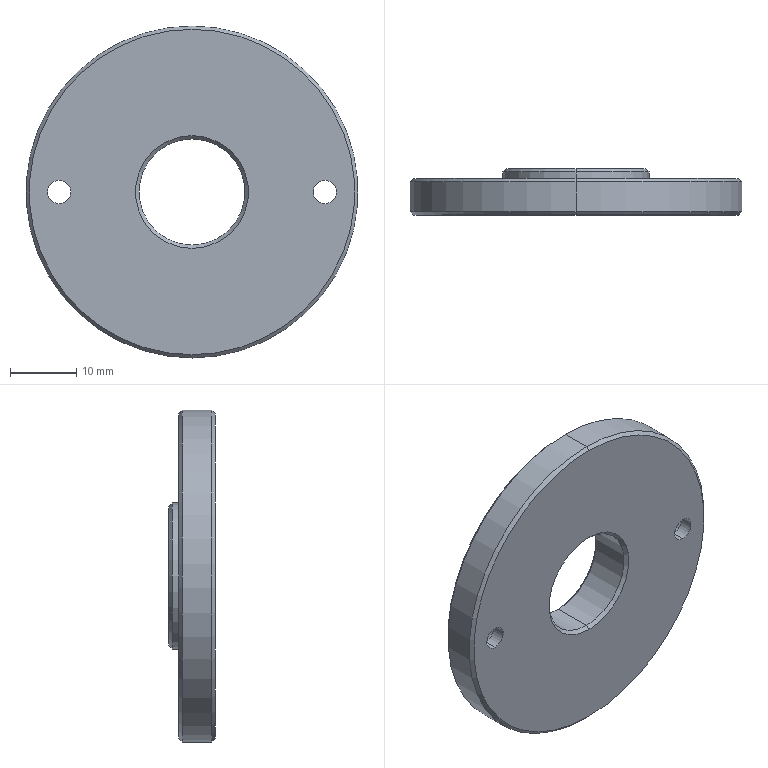Part | SolidWorks | features 3DProfileFeature 1, Chamfer 1, HoleWzd 1, Revolution 1 | 1 solid | 29 faces | box 50 x 7 x 50 mm | volume 9665 mm3 | cylinder 14 | cone 10 | plane 5 | commonest cylinder face diameters 3.5 x4 6 x4 16 x2 22 x2 50 x2
STEP:
#1=CARTESIAN_POINT('',(0.,0.5,8.));
#2=VERTEX_POINT('',#1);
#3=CARTESIAN_POINT('',(0.,0.5,-8.));
#4=VERTEX_POINT('',#3);
#5=CARTESIAN_POINT('',(0.,0.5,0.));
#6=DIRECTION('',(0.,-1.,0.));
#7=DIRECTION('',(0.,0.,1.));
#8=AXIS2_PLACEMENT_3D('',#5,#6,#7);
#9=CIRCLE('',#8,8.);
#10=EDGE_CURVE('',#2,#4,#9,.T.);
#11=ORIENTED_EDGE('',*,*,#10,.F.);
#12=CARTESIAN_POINT('',(0.,0.,8.5));
#13=VERTEX_POINT('',#12);
#14=CARTESIAN_POINT('',(0.,0.,8.5));
#15=DIRECTION('',(0.,-0.7071,0.7071));
#16=VECTOR('',#15,1000.);
#17=LINE('',#14,#16);
#18=EDGE_CURVE('',#2,#13,#17,.T.);
#19=ORIENTED_EDGE('',*,*,#18,.T.);
#20=CARTESIAN_POINT('',(0.,0.,-8.5));
#21=VERTEX_POINT('',#20);
#22=CARTESIAN_POINT('',(0.,0.,0.));
#23=DIRECTION('',(0.,1.,0.));
#24=DIRECTION('',(0.,0.,1.));
#25=AXIS2_PLACEMENT_3D('',#22,#23,#24);
#26=CIRCLE('',#25,8.5);
#27=EDGE_CURVE('',#21,#13,#26,.T.);
#28=ORIENTED_EDGE('',*,*,#27,.F.);
#29=CARTESIAN_POINT('',(0.,0.,-8.5));
#30=DIRECTION('',(0.,-0.7071,-0.7071));
#31=VECTOR('',#30,1000.);
#32=LINE('',#29,#31);
#33=EDGE_CURVE('',#4,#21,#32,.T.);
#34=ORIENTED_EDGE('',*,*,#33,.F.);
#35=EDGE_LOOP('',(#11,#19,#28,#34));
#36=FACE_OUTER_BOUND('',#35,.T.);
#37=CARTESIAN_POINT('',(0.,0.,0.));
#38=DIRECTION('',(0.,-1.,0.));
#39=DIRECTION('',(0.,0.,-1.));
#40=AXIS2_PLACEMENT_3D('',#37,#38,#39);
#41=CONICAL_SURFACE('',#40,8.5,0.7854);
#42=ADVANCED_FACE('',(#36),#41,.F.);
#43=CARTESIAN_POINT('',(0.,6.5,-8.));
#44=VERTEX_POINT('',#43);
#45=CARTESIAN_POINT('',(0.,6.5,8.));
#46=VERTEX_POINT('',#45);
#47=CARTESIAN_POINT('',(0.,6.5,0.));
#48=DIRECTION('',(0.,1.,0.));
#49=DIRECTION('',(0.,0.,-1.));
#50=AXIS2_PLACEMENT_3D('',#47,#48,#49);
#51=CIRCLE('',#50,8.);
#52=EDGE_CURVE('',#44,#46,#51,.T.);
#53=ORIENTED_EDGE('',*,*,#52,.F.);
#54=CARTESIAN_POINT('',(0.,7.,-8.5));
#55=VERTEX_POINT('',#54);
#56=CARTESIAN_POINT('',(0.,6.5,-8.));
#57=DIRECTION('',(0.,0.7071,-0.7071));
#58=VECTOR('',#57,1000.);
#59=LINE('',#56,#58);
#60=EDGE_CURVE('',#44,#55,#59,.T.);
#61=ORIENTED_EDGE('',*,*,#60,.T.);
#62=CARTESIAN_POINT('',(0.,7.,8.5));
#63=VERTEX_POINT('',#62);
#64=CARTESIAN_POINT('',(0.,7.,0.));
#65=DIRECTION('',(0.,-1.,0.));
#66=DIRECTION('',(0.,0.,-1.));
#67=AXIS2_PLACEMENT_3D('',#64,#65,#66);
#68=CIRCLE('',#67,8.5);
#69=EDGE_CURVE('',#63,#55,#68,.T.);
#70=ORIENTED_EDGE('',*,*,#69,.F.);
#71=CARTESIAN_POINT('',(0.,6.5,8.));
#72=DIRECTION('',(0.,0.7071,0.7071));
#73=VECTOR('',#72,1000.);
#74=LINE('',#71,#73);
#75=EDGE_CURVE('',#46,#63,#74,.T.);
#76=ORIENTED_EDGE('',*,*,#75,.F.);
#77=EDGE_LOOP('',(#53,#61,#70,#76));
#78=FACE_OUTER_BOUND('',#77,.T.);
#79=CARTESIAN_POINT('',(0.,6.5,0.));
#80=DIRECTION('',(0.,1.,0.));
#81=DIRECTION('',(0.,0.,1.));
#82=AXIS2_PLACEMENT_3D('',#79,#80,#81);
#83=CONICAL_SURFACE('',#82,8.,0.7854);
#84=ADVANCED_FACE('',(#78),#83,.F.);
#85=CARTESIAN_POINT('',(0.,7.,10.5));
#86=VERTEX_POINT('',#85);
#87=CARTESIAN_POINT('',(0.,7.,-10.5));
#88=VERTEX_POINT('',#87);
#89=CARTESIAN_POINT('',(0.,7.,0.));
#90=DIRECTION('',(0.,1.,0.));
#91=DIRECTION('',(0.,0.,-1.));
#92=AXIS2_PLACEMENT_3D('',#89,#90,#91);
#93=CIRCLE('',#92,10.5);
#94=EDGE_CURVE('',#86,#88,#93,.T.);
#95=ORIENTED_EDGE('',*,*,#94,.F.);
#96=CARTESIAN_POINT('',(0.,6.5,11.));
#97=VERTEX_POINT('',#96);
#98=CARTESIAN_POINT('',(0.,7.,10.5));
#99=DIRECTION('',(0.,-0.7071,0.7071));
#100=VECTOR('',#99,1000.);
#101=LINE('',#98,#100);
#102=EDGE_CURVE('',#86,#97,#101,.T.);
#103=ORIENTED_EDGE('',*,*,#102,.T.);
#104=CARTESIAN_POINT('',(0.,6.5,-11.));
#105=VERTEX_POINT('',#104);
#106=CARTESIAN_POINT('',(0.,6.5,0.));
#107=DIRECTION('',(0.,-1.,0.));
#108=DIRECTION('',(0.,0.,-1.));
#109=AXIS2_PLACEMENT_3D('',#106,#107,#108);
#110=CIRCLE('',#109,11.);
#111=EDGE_CURVE('',#105,#97,#110,.T.);
#112=ORIENTED_EDGE('',*,*,#111,.F.);
#113=CARTESIAN_POINT('',(0.,7.,-10.5));
#114=DIRECTION('',(0.,-0.7071,-0.7071));
#115=VECTOR('',#114,1000.);
#116=LINE('',#113,#115);
#117=EDGE_CURVE('',#88,#105,#116,.T.);
#118=ORIENTED_EDGE('',*,*,#117,.F.);
#119=EDGE_LOOP('',(#95,#103,#112,#118));
#120=FACE_OUTER_BOUND('',#119,.T.);
#121=CARTESIAN_POINT('',(0.,7.,0.));
#122=DIRECTION('',(0.,-1.,0.));
#123=DIRECTION('',(0.,0.,-1.));
#124=AXIS2_PLACEMENT_3D('',#121,#122,#123);
#125=CONICAL_SURFACE('',#124,10.5,0.7854);
#126=ADVANCED_FACE('',(#120),#125,.T.);
#127=CARTESIAN_POINT('',(0.,5.5,24.5));
#128=VERTEX_POINT('',#127);
#129=CARTESIAN_POINT('',(0.,5.5,-24.5));
#130=VERTEX_POINT('',#129);
#131=CARTESIAN_POINT('',(0.,5.5,0.));
#132=DIRECTION('',(0.,1.,0.));
#133=DIRECTION('',(0.,0.,-1.));
#134=AXIS2_PLACEMENT_3D('',#131,#132,#133);
#135=CIRCLE('',#134,24.5);
#136=EDGE_CURVE('',#128,#130,#135,.T.);
#137=ORIENTED_EDGE('',*,*,#136,.F.);
#138=CARTESIAN_POINT('',(0.,5.,25.));
#139=VERTEX_POINT('',#138);
#140=CARTESIAN_POINT('',(0.,5.5,24.5));
#141=DIRECTION('',(0.,-0.7071,0.7071));
#142=VECTOR('',#141,1000.);
#143=LINE('',#140,#142);
#144=EDGE_CURVE('',#128,#139,#143,.T.);
#145=ORIENTED_EDGE('',*,*,#144,.T.);
#146=CARTESIAN_POINT('',(0.,5.,-25.));
#147=VERTEX_POINT('',#146);
#148=CARTESIAN_POINT('',(0.,5.,0.));
#149=DIRECTION('',(0.,-1.,0.));
#150=DIRECTION('',(0.,0.,-1.));
#151=AXIS2_PLACEMENT_3D('',#148,#149,#150);
#152=CIRCLE('',#151,25.);
#153=EDGE_CURVE('',#147,#139,#152,.T.);
#154=ORIENTED_EDGE('',*,*,#153,.F.);
#155=CARTESIAN_POINT('',(0.,5.5,-24.5));
#156=DIRECTION('',(0.,-0.7071,-0.7071));
#157=VECTOR('',#156,1000.);
#158=LINE('',#155,#157);
#159=EDGE_CURVE('',#130,#147,#158,.T.);
#160=ORIENTED_EDGE('',*,*,#159,.F.);
#161=EDGE_LOOP('',(#137,#145,#154,#160));
#162=FACE_OUTER_BOUND('',#161,.T.);
#163=CARTESIAN_POINT('',(0.,5.5,0.));
#164=DIRECTION('',(0.,-1.,0.));
#165=DIRECTION('',(0.,0.,-1.));
#166=AXIS2_PLACEMENT_3D('',#163,#164,#165);
#167=CONICAL_SURFACE('',#166,24.5,0.7854);
#168=ADVANCED_FACE('',(#162),#167,.T.);
#169=CARTESIAN_POINT('',(0.,0.,-24.5));
#170=VERTEX_POINT('',#169);
#171=CARTESIAN_POINT('',(0.,0.,24.5));
#172=VERTEX_POINT('',#171);
#173=CARTESIAN_POINT('',(0.,0.,0.));
#174=DIRECTION('',(0.,-1.,0.));
#175=DIRECTION('',(0.,0.,1.));
#176=AXIS2_PLACEMENT_3D('',#173,#174,#175);
#177=CIRCLE('',#176,24.5);
#178=EDGE_CURVE('',#170,#172,#177,.T.);
#179=ORIENTED_EDGE('',*,*,#178,.F.);
#180=CARTESIAN_POINT('',(0.,0.5,-25.));
#181=VERTEX_POINT('',#180);
#182=CARTESIAN_POINT('',(0.,0.5,-25.));
#183=DIRECTION('',(0.,0.7071,-0.7071));
#184=VECTOR('',#183,1000.);
#185=LINE('',#182,#184);
#186=EDGE_CURVE('',#170,#181,#185,.T.);
#187=ORIENTED_EDGE('',*,*,#186,.T.);
#188=CARTESIAN_POINT('',(0.,0.5,25.));
#189=VERTEX_POINT('',#188);
#190=CARTESIAN_POINT('',(0.,0.5,0.));
#191=DIRECTION('',(0.,1.,0.));
#192=DIRECTION('',(0.,0.,1.));
#193=AXIS2_PLACEMENT_3D('',#190,#191,#192);
#194=CIRCLE('',#193,25.);
#195=EDGE_CURVE('',#189,#181,#194,.T.);
#196=ORIENTED_EDGE('',*,*,#195,.F.);
#197=CARTESIAN_POINT('',(0.,0.5,25.));
#198=DIRECTION('',(0.,0.7071,0.7071));
#199=VECTOR('',#198,1000.);
#200=LINE('',#197,#199);
#201=EDGE_CURVE('',#172,#189,#200,.T.);
#202=ORIENTED_EDGE('',*,*,#201,.F.);
#203=EDGE_LOOP('',(#179,#187,#196,#202));
#204=FACE_OUTER_BOUND('',#203,.T.);
#205=CARTESIAN_POINT('',(0.,0.5,0.));
#206=DIRECTION('',(0.,1.,0.));
#207=DIRECTION('',(0.,0.,1.));
#208=AXIS2_PLACEMENT_3D('',#205,#206,#207);
#209=CONICAL_SURFACE('',#208,25.,0.7854);
#210=ADVANCED_FACE('',(#204),#209,.T.);
#211=CARTESIAN_POINT('',(-20.,2.,-3.));
#212=VERTEX_POINT('',#211);
#213=CARTESIAN_POINT('',(-20.,2.,3.));
#214=VERTEX_POINT('',#213);
#215=CARTESIAN_POINT('',(-20.,2.,0.));
#216=DIRECTION('',(0.,1.,0.));
#217=DIRECTION('',(0.,0.,1.));
#218=AXIS2_PLACEMENT_3D('',#215,#216,#217);
#219=CIRCLE('',#218,3.);
#220=EDGE_CURVE('',#212,#214,#219,.T.);
#221=ORIENTED_EDGE('',*,*,#220,.F.);
#222=CARTESIAN_POINT('',(-20.,5.5,-3.));
#223=VERTEX_POINT('',#222);
#224=CARTESIAN_POINT('',(-20.,5.5,-3.));
#225=DIRECTION('',(0.,1.,0.));
#226=VECTOR('',#225,1000.);
#227=LINE('',#224,#226);
#228=EDGE_CURVE('',#212,#223,#227,.T.);
#229=ORIENTED_EDGE('',*,*,#228,.T.);
#230=CARTESIAN_POINT('',(-20.,5.5,3.));
#231=VERTEX_POINT('',#230);
#232=CARTESIAN_POINT('',(-20.,5.5,0.));
#233=DIRECTION('',(0.,1.,0.));
#234=DIRECTION('',(0.,0.,1.));
#235=AXIS2_PLACEMENT_3D('',#232,#233,#234);
#236=CIRCLE('',#235,3.);
#237=EDGE_CURVE('',#223,#231,#236,.T.);
#238=ORIENTED_EDGE('',*,*,#237,.T.);
#239=CARTESIAN_POINT('',(-20.,5.5,3.));
#240=DIRECTION('',(0.,1.,0.));
#241=VECTOR('',#240,1000.);
#242=LINE('',#239,#241);
#243=EDGE_CURVE('',#214,#231,#242,.T.);
#244=ORIENTED_EDGE('',*,*,#243,.F.);
#245=EDGE_LOOP('',(#221,#229,#238,#244));
#246=FACE_OUTER_BOUND('',#245,.T.);
#247=CARTESIAN_POINT('',(-20.,5.5,0.));
#248=DIRECTION('',(0.,1.,0.));
#249=DIRECTION('',(0.,0.,1.));
#250=AXIS2_PLACEMENT_3D('',#247,#248,#249);
#251=CYLINDRICAL_SURFACE('',#250,3.);
#252=ADVANCED_FACE('',(#246),#251,.F.);
#253=CARTESIAN_POINT('',(-20.,0.,-1.75));
#254=VERTEX_POINT('',#253);
#255=CARTESIAN_POINT('',(-20.,0.,1.75));
#256=VERTEX_POINT('',#255);
#257=CARTESIAN_POINT('',(-20.,0.,0.));
#258=DIRECTION('',(0.,1.,0.));
#259=DIRECTION('',(0.,0.,1.));
#260=AXIS2_PLACEMENT_3D('',#257,#258,#259);
#261=CIRCLE('',#260,1.75);
#262=EDGE_CURVE('',#254,#256,#261,.T.);
#263=ORIENTED_EDGE('',*,*,#262,.F.);
#264=CARTESIAN_POINT('',(-20.,2.,-1.75));
#265=VERTEX_POINT('',#264);
#266=CARTESIAN_POINT('',(-20.,5.5,-1.75));
#267=DIRECTION('',(0.,1.,0.));
#268=VECTOR('',#267,1000.);
#269=LINE('',#266,#268);
#270=EDGE_CURVE('',#254,#265,#269,.T.);
#271=ORIENTED_EDGE('',*,*,#270,.T.);
#272=CARTESIAN_POINT('',(-20.,2.,1.75));
#273=VERTEX_POINT('',#272);
#274=CARTESIAN_POINT('',(-20.,2.,0.));
#275=DIRECTION('',(0.,1.,0.));
#276=DIRECTION('',(0.,0.,1.));
#277=AXIS2_PLACEMENT_3D('',#274,#275,#276);
#278=CIRCLE('',#277,1.75);
#279=EDGE_CURVE('',#265,#273,#278,.T.);
#280=ORIENTED_EDGE('',*,*,#279,.T.);
#281=CARTESIAN_POINT('',(-20.,5.5,1.75));
#282=DIRECTION('',(0.,1.,0.));
#283=VECTOR('',#282,1000.);
#284=LINE('',#281,#283);
#285=EDGE_CURVE('',#256,#273,#284,.T.);
#286=ORIENTED_EDGE('',*,*,#285,.F.);
#287=EDGE_LOOP('',(#263,#271,#280,#286));
#288=FACE_OUTER_BOUND('',#287,.T.);
#289=CARTESIAN_POINT('',(-20.,5.5,0.));
#290=DIRECTION('',(0.,1.,0.));
#291=DIRECTION('',(0.,0.,1.));
#292=AXIS2_PLACEMENT_3D('',#289,#290,#291);
#293=CYLINDRICAL_SURFACE('',#292,1.75);
#294=ADVANCED_FACE('',(#288),#293,.F.);
#295=CARTESIAN_POINT('',(20.,2.,-3.));
#296=VERTEX_POINT('',#295);
#297=CARTESIAN_POINT('',(20.,2.,3.));
#298=VERTEX_POINT('',#297);
#299=CARTESIAN_POINT('',(20.,2.,0.));
#300=DIRECTION('',(0.,1.,0.));
#301=DIRECTION('',(0.,0.,1.));
#302=AXIS2_PLACEMENT_3D('',#299,#300,#301);
#303=CIRCLE('',#302,3.);
#304=EDGE_CURVE('',#296,#298,#303,.T.);
#305=ORIENTED_EDGE('',*,*,#304,.F.);
#306=CARTESIAN_POINT('',(20.,5.5,-3.));
#307=VERTEX_POINT('',#306);
#308=CARTESIAN_POINT('',(20.,5.5,-3.));
#309=DIRECTION('',(0.,1.,0.));
#310=VECTOR('',#309,1000.);
#311=LINE('',#308,#310);
#312=EDGE_CURVE('',#296,#307,#311,.T.);
#313=ORIENTED_EDGE('',*,*,#312,.T.);
#314=CARTESIAN_POINT('',(20.,5.5,3.));
#315=VERTEX_POINT('',#314);
#316=CARTESIAN_POINT('',(20.,5.5,0.));
#317=DIRECTION('',(0.,1.,0.));
#318=DIRECTION('',(0.,0.,1.));
#319=AXIS2_PLACEMENT_3D('',#316,#317,#318);
#320=CIRCLE('',#319,3.);
#321=EDGE_CURVE('',#307,#315,#320,.T.);
#322=ORIENTED_EDGE('',*,*,#321,.T.);
#323=CARTESIAN_POINT('',(20.,5.5,3.));
#324=DIRECTION('',(0.,1.,0.));
#325=VECTOR('',#324,1000.);
#326=LINE('',#323,#325);
#327=EDGE_CURVE('',#298,#315,#326,.T.);
#328=ORIENTED_EDGE('',*,*,#327,.F.);
#329=EDGE_LOOP('',(#305,#313,#322,#328));
#330=FACE_OUTER_BOUND('',#329,.T.);
#331=CARTESIAN_POINT('',(20.,5.5,0.));
#332=DIRECTION('',(0.,1.,0.));
#333=DIRECTION('',(0.,0.,1.));
#334=AXIS2_PLACEMENT_3D('',#331,#332,#333);
#335=CYLINDRICAL_SURFACE('',#334,3.);
#336=ADVANCED_FACE('',(#330),#335,.F.);
#337=CARTESIAN_POINT('',(20.,0.,-1.75));
#338=VERTEX_POINT('',#337);
#339=CARTESIAN_POINT('',(20.,0.,1.75));
#340=VERTEX_POINT('',#339);
#341=CARTESIAN_POINT('',(20.,0.,0.));
#342=DIRECTION('',(0.,1.,0.));
#343=DIRECTION('',(0.,0.,1.));
#344=AXIS2_PLACEMENT_3D('',#341,#342,#343);
#345=CIRCLE('',#344,1.75);
#346=EDGE_CURVE('',#338,#340,#345,.T.);
#347=ORIENTED_EDGE('',*,*,#346,.F.);
#348=CARTESIAN_POINT('',(20.,2.,-1.75));
#349=VERTEX_POINT('',#348);
#350=CARTESIAN_POINT('',(20.,5.5,-1.75));
#351=DIRECTION('',(0.,1.,0.));
#352=VECTOR('',#351,1000.);
#353=LINE('',#350,#352);
#354=EDGE_CURVE('',#338,#349,#353,.T.);
#355=ORIENTED_EDGE('',*,*,#354,.T.);
#356=CARTESIAN_POINT('',(20.,2.,1.75));
#357=VERTEX_POINT('',#356);
#358=CARTESIAN_POINT('',(20.,2.,0.));
#359=DIRECTION('',(0.,1.,0.));
#360=DIRECTION('',(0.,0.,1.));
#361=AXIS2_PLACEMENT_3D('',#358,#359,#360);
#362=CIRCLE('',#361,1.75);
#363=EDGE_CURVE('',#349,#357,#362,.T.);
#364=ORIENTED_EDGE('',*,*,#363,.T.);
#365=CARTESIAN_POINT('',(20.,5.5,1.75));
#366=DIRECTION('',(0.,1.,0.));
#367=VECTOR('',#366,1000.);
#368=LINE('',#365,#367);
#369=EDGE_CURVE('',#340,#357,#368,.T.);
#370=ORIENTED_EDGE('',*,*,#369,.F.);
#371=EDGE_LOOP('',(#347,#355,#364,#370));
#372=FACE_OUTER_BOUND('',#371,.T.);
#373=CARTESIAN_POINT('',(20.,5.5,0.));
#374=DIRECTION('',(0.,1.,0.));
#375=DIRECTION('',(0.,0.,1.));
#376=AXIS2_PLACEMENT_3D('',#373,#374,#375);
#377=CYLINDRICAL_SURFACE('',#376,1.75);
#378=ADVANCED_FACE('',(#372),#377,.F.);
#379=ORIENTED_EDGE('',*,*,#10,.T.);
#380=CARTESIAN_POINT('',(0.,21.458,-8.));
#381=DIRECTION('',(0.,1.,0.));
#382=VECTOR('',#381,1000.);
#383=LINE('',#380,#382);
#384=EDGE_CURVE('',#4,#44,#383,.T.);
#385=ORIENTED_EDGE('',*,*,#384,.T.);
#386=ORIENTED_EDGE('',*,*,#52,.T.);
#387=CARTESIAN_POINT('',(0.,21.458,8.));
#388=DIRECTION('',(0.,1.,0.));
#389=VECTOR('',#388,1000.);
#390=LINE('',#387,#389);
#391=EDGE_CURVE('',#2,#46,#390,.T.);
#392=ORIENTED_EDGE('',*,*,#391,.F.);
#393=EDGE_LOOP('',(#379,#385,#386,#392));
#394=FACE_OUTER_BOUND('',#393,.T.);
#395=CARTESIAN_POINT('',(0.,21.458,0.));
#396=DIRECTION('',(0.,1.,0.));
#397=DIRECTION('',(0.,0.,1.));
#398=AXIS2_PLACEMENT_3D('',#395,#396,#397);
#399=CYLINDRICAL_SURFACE('',#398,8.);
#400=ADVANCED_FACE('',(#394),#399,.F.);
#401=CARTESIAN_POINT('',(0.,5.5,11.));
#402=VERTEX_POINT('',#401);
#403=CARTESIAN_POINT('',(0.,5.5,-11.));
#404=VERTEX_POINT('',#403);
#405=CARTESIAN_POINT('',(0.,5.5,0.));
#406=DIRECTION('',(0.,1.,0.));
#407=DIRECTION('',(0.,0.,1.));
#408=AXIS2_PLACEMENT_3D('',#405,#406,#407);
#409=CIRCLE('',#408,11.);
#410=EDGE_CURVE('',#402,#404,#409,.T.);
#411=ORIENTED_EDGE('',*,*,#410,.T.);
#412=CARTESIAN_POINT('',(0.,21.458,-11.));
#413=DIRECTION('',(0.,1.,0.));
#414=VECTOR('',#413,1000.);
#415=LINE('',#412,#414);
#416=EDGE_CURVE('',#404,#105,#415,.T.);
#417=ORIENTED_EDGE('',*,*,#416,.T.);
#418=ORIENTED_EDGE('',*,*,#111,.T.);
#419=CARTESIAN_POINT('',(0.,21.458,11.));
#420=DIRECTION('',(0.,1.,0.));
#421=VECTOR('',#420,1000.);
#422=LINE('',#419,#421);
#423=EDGE_CURVE('',#402,#97,#422,.T.);
#424=ORIENTED_EDGE('',*,*,#423,.F.);
#425=EDGE_LOOP('',(#411,#417,#418,#424));
#426=FACE_OUTER_BOUND('',#425,.T.);
#427=CARTESIAN_POINT('',(0.,21.458,0.));
#428=DIRECTION('',(0.,1.,0.));
#429=DIRECTION('',(0.,0.,1.));
#430=AXIS2_PLACEMENT_3D('',#427,#428,#429);
#431=CYLINDRICAL_SURFACE('',#430,11.);
#432=ADVANCED_FACE('',(#426),#431,.T.);
#433=ORIENTED_EDGE('',*,*,#195,.T.);
#434=CARTESIAN_POINT('',(0.,21.458,-25.));
#435=DIRECTION('',(0.,1.,0.));
#436=VECTOR('',#435,1000.);
#437=LINE('',#434,#436);
#438=EDGE_CURVE('',#181,#147,#437,.T.);
#439=ORIENTED_EDGE('',*,*,#438,.T.);
#440=ORIENTED_EDGE('',*,*,#153,.T.);
#441=CARTESIAN_POINT('',(0.,21.458,25.));
#442=DIRECTION('',(0.,1.,0.));
#443=VECTOR('',#442,1000.);
#444=LINE('',#441,#443);
#445=EDGE_CURVE('',#189,#139,#444,.T.);
#446=ORIENTED_EDGE('',*,*,#445,.F.);
#447=EDGE_LOOP('',(#433,#439,#440,#446));
#448=FACE_OUTER_BOUND('',#447,.T.);
#449=CARTESIAN_POINT('',(0.,21.458,0.));
#450=DIRECTION('',(0.,1.,0.));
#451=DIRECTION('',(0.,0.,1.));
#452=AXIS2_PLACEMENT_3D('',#449,#450,#451);
#453=CYLINDRICAL_SURFACE('',#452,25.);
#454=ADVANCED_FACE('',(#448),#453,.T.);
#455=CARTESIAN_POINT('',(0.,5.5,0.));
#456=DIRECTION('',(0.,1.,0.));
#457=DIRECTION('',(0.,0.,-1.));
#458=AXIS2_PLACEMENT_3D('',#455,#456,#457);
#459=CIRCLE('',#458,24.5);
#460=EDGE_CURVE('',#130,#128,#459,.T.);
#461=ORIENTED_EDGE('',*,*,#460,.T.);
#462=ORIENTED_EDGE('',*,*,#136,.T.);
#463=EDGE_LOOP('',(#461,#462));
#464=FACE_OUTER_BOUND('',#463,.T.);
#465=ORIENTED_EDGE('',*,*,#410,.F.);
#466=CARTESIAN_POINT('',(0.,5.5,0.));
#467=DIRECTION('',(0.,1.,0.));
#468=DIRECTION('',(0.,0.,1.));
#469=AXIS2_PLACEMENT_3D('',#466,#467,#468);
#470=CIRCLE('',#469,11.);
#471=EDGE_CURVE('',#404,#402,#470,.T.);
#472=ORIENTED_EDGE('',*,*,#471,.F.);
#473=EDGE_LOOP('',(#465,#472));
#474=FACE_BOUND('',#473,.T.);
#475=CARTESIAN_POINT('',(20.,5.5,0.));
#476=DIRECTION('',(0.,1.,0.));
#477=DIRECTION('',(0.,0.,1.));
#478=AXIS2_PLACEMENT_3D('',#475,#476,#477);
#479=CIRCLE('',#478,3.);
#480=EDGE_CURVE('',#315,#307,#479,.T.);
#481=ORIENTED_EDGE('',*,*,#480,.F.);
#482=ORIENTED_EDGE('',*,*,#321,.F.);
#483=EDGE_LOOP('',(#481,#482));
#484=FACE_BOUND('',#483,.T.);
#485=CARTESIAN_POINT('',(-20.,5.5,0.));
#486=DIRECTION('',(0.,1.,0.));
#487=DIRECTION('',(0.,0.,1.));
#488=AXIS2_PLACEMENT_3D('',#485,#486,#487);
#489=CIRCLE('',#488,3.);
#490=EDGE_CURVE('',#231,#223,#489,.T.);
#491=ORIENTED_EDGE('',*,*,#490,.F.);
#492=ORIENTED_EDGE('',*,*,#237,.F.);
#493=EDGE_LOOP('',(#491,#492));
#494=FACE_BOUND('',#493,.T.);
#495=CARTESIAN_POINT('',(25.,5.5,0.));
#496=DIRECTION('',(0.,-1.,0.));
#497=DIRECTION('',(0.,0.,-1.));
#498=AXIS2_PLACEMENT_3D('',#495,#496,#497);
#499=PLANE('',#498);
#500=ADVANCED_FACE('',(#464,#474,#484,#494),#499,.F.);
#501=ORIENTED_EDGE('',*,*,#438,.F.);
#502=CARTESIAN_POINT('',(0.,0.5,0.));
#503=DIRECTION('',(0.,1.,0.));
#504=DIRECTION('',(0.,0.,1.));
#505=AXIS2_PLACEMENT_3D('',#502,#503,#504);
#506=CIRCLE('',#505,25.);
#507=EDGE_CURVE('',#181,#189,#506,.T.);
#508=ORIENTED_EDGE('',*,*,#507,.T.);
#509=ORIENTED_EDGE('',*,*,#445,.T.);
#510=CARTESIAN_POINT('',(0.,5.,0.));
#511=DIRECTION('',(0.,-1.,0.));
#512=DIRECTION('',(0.,0.,-1.));
#513=AXIS2_PLACEMENT_3D('',#510,#511,#512);
#514=CIRCLE('',#513,25.);
#515=EDGE_CURVE('',#139,#147,#514,.T.);
#516=ORIENTED_EDGE('',*,*,#515,.T.);
#517=EDGE_LOOP('',(#501,#508,#509,#516));
#518=FACE_OUTER_BOUND('',#517,.T.);
#519=CARTESIAN_POINT('',(0.,21.458,0.));
#520=DIRECTION('',(0.,1.,0.));
#521=DIRECTION('',(0.,0.,1.));
#522=AXIS2_PLACEMENT_3D('',#519,#520,#521);
#523=CYLINDRICAL_SURFACE('',#522,25.);
#524=ADVANCED_FACE('',(#518),#523,.T.);
#525=ORIENTED_EDGE('',*,*,#416,.F.);
#526=ORIENTED_EDGE('',*,*,#471,.T.);
#527=ORIENTED_EDGE('',*,*,#423,.T.);
#528=CARTESIAN_POINT('',(0.,6.5,0.));
#529=DIRECTION('',(0.,-1.,0.));
#530=DIRECTION('',(0.,0.,-1.));
#531=AXIS2_PLACEMENT_3D('',#528,#529,#530);
#532=CIRCLE('',#531,11.);
#533=EDGE_CURVE('',#97,#105,#532,.T.);
#534=ORIENTED_EDGE('',*,*,#533,.T.);
#535=EDGE_LOOP('',(#525,#526,#527,#534));
#536=FACE_OUTER_BOUND('',#535,.T.);
#537=CARTESIAN_POINT('',(0.,21.458,0.));
#538=DIRECTION('',(0.,1.,0.));
#539=DIRECTION('',(0.,0.,1.));
#540=AXIS2_PLACEMENT_3D('',#537,#538,#539);
#541=CYLINDRICAL_SURFACE('',#540,11.);
#542=ADVANCED_FACE('',(#536),#541,.T.);
#543=CARTESIAN_POINT('',(0.,7.,0.));
#544=DIRECTION('',(0.,1.,0.));
#545=DIRECTION('',(0.,0.,-1.));
#546=AXIS2_PLACEMENT_3D('',#543,#544,#545);
#547=CIRCLE('',#546,10.5);
#548=EDGE_CURVE('',#88,#86,#547,.T.);
#549=ORIENTED_EDGE('',*,*,#548,.T.);
#550=ORIENTED_EDGE('',*,*,#94,.T.);
#551=EDGE_LOOP('',(#549,#550));
#552=FACE_OUTER_BOUND('',#551,.T.);
#553=ORIENTED_EDGE('',*,*,#69,.T.);
#554=CARTESIAN_POINT('',(0.,7.,0.));
#555=DIRECTION('',(0.,-1.,0.));
#556=DIRECTION('',(0.,0.,-1.));
#557=AXIS2_PLACEMENT_3D('',#554,#555,#556);
#558=CIRCLE('',#557,8.5);
#559=EDGE_CURVE('',#55,#63,#558,.T.);
#560=ORIENTED_EDGE('',*,*,#559,.T.);
#561=EDGE_LOOP('',(#553,#560));
#562=FACE_BOUND('',#561,.T.);
#563=CARTESIAN_POINT('',(11.,7.,0.));
#564=DIRECTION('',(0.,-1.,0.));
#565=DIRECTION('',(0.,0.,-1.));
#566=AXIS2_PLACEMENT_3D('',#563,#564,#565);
#567=PLANE('',#566);
#568=ADVANCED_FACE('',(#552,#562),#567,.F.);
#569=ORIENTED_EDGE('',*,*,#384,.F.);
#570=CARTESIAN_POINT('',(0.,0.5,0.));
#571=DIRECTION('',(0.,-1.,0.));
#572=DIRECTION('',(0.,0.,1.));
#573=AXIS2_PLACEMENT_3D('',#570,#571,#572);
#574=CIRCLE('',#573,8.);
#575=EDGE_CURVE('',#4,#2,#574,.T.);
#576=ORIENTED_EDGE('',*,*,#575,.T.);
#577=ORIENTED_EDGE('',*,*,#391,.T.);
#578=CARTESIAN_POINT('',(0.,6.5,0.));
#579=DIRECTION('',(0.,1.,0.));
#580=DIRECTION('',(0.,0.,-1.));
#581=AXIS2_PLACEMENT_3D('',#578,#579,#580);
#582=CIRCLE('',#581,8.);
#583=EDGE_CURVE('',#46,#44,#582,.T.);
#584=ORIENTED_EDGE('',*,*,#583,.T.);
#585=EDGE_LOOP('',(#569,#576,#577,#584));
#586=FACE_OUTER_BOUND('',#585,.T.);
#587=CARTESIAN_POINT('',(0.,21.458,0.));
#588=DIRECTION('',(0.,1.,0.));
#589=DIRECTION('',(0.,0.,1.));
#590=AXIS2_PLACEMENT_3D('',#587,#588,#589);
#591=CYLINDRICAL_SURFACE('',#590,8.);
#592=ADVANCED_FACE('',(#586),#591,.F.);
#593=CARTESIAN_POINT('',(0.,0.,0.));
#594=DIRECTION('',(0.,-1.,0.));
#595=DIRECTION('',(0.,0.,1.));
#596=AXIS2_PLACEMENT_3D('',#593,#594,#595);
#597=CIRCLE('',#596,24.5);
#598=EDGE_CURVE('',#172,#170,#597,.T.);
#599=ORIENTED_EDGE('',*,*,#598,.T.);
#600=ORIENTED_EDGE('',*,*,#178,.T.);
#601=EDGE_LOOP('',(#599,#600));
#602=FACE_OUTER_BOUND('',#601,.T.);
#603=ORIENTED_EDGE('',*,*,#27,.T.);
#604=CARTESIAN_POINT('',(0.,0.,0.));
#605=DIRECTION('',(0.,1.,0.));
#606=DIRECTION('',(0.,0.,1.));
#607=AXIS2_PLACEMENT_3D('',#604,#605,#606);
#608=CIRCLE('',#607,8.5);
#609=EDGE_CURVE('',#13,#21,#608,.T.);
#610=ORIENTED_EDGE('',*,*,#609,.T.);
#611=EDGE_LOOP('',(#603,#610));
#612=FACE_BOUND('',#611,.T.);
#613=CARTESIAN_POINT('',(-20.,0.,0.));
#614=DIRECTION('',(0.,1.,0.));
#615=DIRECTION('',(0.,0.,1.));
#616=AXIS2_PLACEMENT_3D('',#613,#614,#615);
#617=CIRCLE('',#616,1.75);
#618=EDGE_CURVE('',#256,#254,#617,.T.);
#619=ORIENTED_EDGE('',*,*,#618,.T.);
#620=ORIENTED_EDGE('',*,*,#262,.T.);
#621=EDGE_LOOP('',(#619,#620));
#622=FACE_BOUND('',#621,.T.);
#623=CARTESIAN_POINT('',(20.,0.,0.));
#624=DIRECTION('',(0.,1.,0.));
#625=DIRECTION('',(0.,0.,1.));
#626=AXIS2_PLACEMENT_3D('',#623,#624,#625);
#627=CIRCLE('',#626,1.75);
#628=EDGE_CURVE('',#340,#338,#627,.T.);
#629=ORIENTED_EDGE('',*,*,#628,.T.);
#630=ORIENTED_EDGE('',*,*,#346,.T.);
#631=EDGE_LOOP('',(#629,#630));
#632=FACE_BOUND('',#631,.T.);
#633=CARTESIAN_POINT('',(8.,0.,0.));
#634=DIRECTION('',(0.,1.,0.));
#635=DIRECTION('',(0.,0.,1.));
#636=AXIS2_PLACEMENT_3D('',#633,#634,#635);
#637=PLANE('',#636);
#638=ADVANCED_FACE('',(#602,#612,#622,#632),#637,.F.);
#639=ORIENTED_EDGE('',*,*,#354,.F.);
#640=ORIENTED_EDGE('',*,*,#628,.F.);
#641=ORIENTED_EDGE('',*,*,#369,.T.);
#642=CARTESIAN_POINT('',(20.,2.,0.));
#643=DIRECTION('',(0.,1.,0.));
#644=DIRECTION('',(0.,0.,1.));
#645=AXIS2_PLACEMENT_3D('',#642,#643,#644);
#646=CIRCLE('',#645,1.75);
#647=EDGE_CURVE('',#357,#349,#646,.T.);
#648=ORIENTED_EDGE('',*,*,#647,.T.);
#649=EDGE_LOOP('',(#639,#640,#641,#648));
#650=FACE_OUTER_BOUND('',#649,.T.);
#651=CARTESIAN_POINT('',(20.,5.5,0.));
#652=DIRECTION('',(0.,1.,0.));
#653=DIRECTION('',(0.,0.,1.));
#654=AXIS2_PLACEMENT_3D('',#651,#652,#653);
#655=CYLINDRICAL_SURFACE('',#654,1.75);
#656=ADVANCED_FACE('',(#650),#655,.F.);
#657=ORIENTED_EDGE('',*,*,#647,.F.);
#658=ORIENTED_EDGE('',*,*,#363,.F.);
#659=EDGE_LOOP('',(#657,#658));
#660=FACE_BOUND('',#659,.T.);
#661=CARTESIAN_POINT('',(20.,2.,0.));
#662=DIRECTION('',(0.,1.,0.));
#663=DIRECTION('',(0.,0.,1.));
#664=AXIS2_PLACEMENT_3D('',#661,#662,#663);
#665=CIRCLE('',#664,3.);
#666=EDGE_CURVE('',#298,#296,#665,.T.);
#667=ORIENTED_EDGE('',*,*,#666,.T.);
#668=ORIENTED_EDGE('',*,*,#304,.T.);
#669=EDGE_LOOP('',(#667,#668));
#670=FACE_OUTER_BOUND('',#669,.T.);
#671=CARTESIAN_POINT('',(21.75,2.,0.));
#672=DIRECTION('',(0.,-1.,0.));
#673=DIRECTION('',(0.,0.,-1.));
#674=AXIS2_PLACEMENT_3D('',#671,#672,#673);
#675=PLANE('',#674);
#676=ADVANCED_FACE('',(#660,#670),#675,.F.);
#677=ORIENTED_EDGE('',*,*,#312,.F.);
#678=ORIENTED_EDGE('',*,*,#666,.F.);
#679=ORIENTED_EDGE('',*,*,#327,.T.);
#680=ORIENTED_EDGE('',*,*,#480,.T.);
#681=EDGE_LOOP('',(#677,#678,#679,#680));
#682=FACE_OUTER_BOUND('',#681,.T.);
#683=CARTESIAN_POINT('',(20.,5.5,0.));
#684=DIRECTION('',(0.,1.,0.));
#685=DIRECTION('',(0.,0.,1.));
#686=AXIS2_PLACEMENT_3D('',#683,#684,#685);
#687=CYLINDRICAL_SURFACE('',#686,3.);
#688=ADVANCED_FACE('',(#682),#687,.F.);
#689=ORIENTED_EDGE('',*,*,#270,.F.);
#690=ORIENTED_EDGE('',*,*,#618,.F.);
#691=ORIENTED_EDGE('',*,*,#285,.T.);
#692=CARTESIAN_POINT('',(-20.,2.,0.));
#693=DIRECTION('',(0.,1.,0.));
#694=DIRECTION('',(0.,0.,1.));
#695=AXIS2_PLACEMENT_3D('',#692,#693,#694);
#696=CIRCLE('',#695,1.75);
#697=EDGE_CURVE('',#273,#265,#696,.T.);
#698=ORIENTED_EDGE('',*,*,#697,.T.);
#699=EDGE_LOOP('',(#689,#690,#691,#698));
#700=FACE_OUTER_BOUND('',#699,.T.);
#701=CARTESIAN_POINT('',(-20.,5.5,0.));
#702=DIRECTION('',(0.,1.,0.));
#703=DIRECTION('',(0.,0.,1.));
#704=AXIS2_PLACEMENT_3D('',#701,#702,#703);
#705=CYLINDRICAL_SURFACE('',#704,1.75);
#706=ADVANCED_FACE('',(#700),#705,.F.);
#707=ORIENTED_EDGE('',*,*,#697,.F.);
#708=ORIENTED_EDGE('',*,*,#279,.F.);
#709=EDGE_LOOP('',(#707,#708));
#710=FACE_BOUND('',#709,.T.);
#711=CARTESIAN_POINT('',(-20.,2.,0.));
#712=DIRECTION('',(0.,1.,0.));
#713=DIRECTION('',(0.,0.,1.));
#714=AXIS2_PLACEMENT_3D('',#711,#712,#713);
#715=CIRCLE('',#714,3.);
#716=EDGE_CURVE('',#214,#212,#715,.T.);
#717=ORIENTED_EDGE('',*,*,#716,.T.);
#718=ORIENTED_EDGE('',*,*,#220,.T.);
#719=EDGE_LOOP('',(#717,#718));
#720=FACE_OUTER_BOUND('',#719,.T.);
#721=CARTESIAN_POINT('',(-18.25,2.,0.));
#722=DIRECTION('',(0.,-1.,0.));
#723=DIRECTION('',(0.,0.,-1.));
#724=AXIS2_PLACEMENT_3D('',#721,#722,#723);
#725=PLANE('',#724);
#726=ADVANCED_FACE('',(#710,#720),#725,.F.);
#727=ORIENTED_EDGE('',*,*,#228,.F.);
#728=ORIENTED_EDGE('',*,*,#716,.F.);
#729=ORIENTED_EDGE('',*,*,#243,.T.);
#730=ORIENTED_EDGE('',*,*,#490,.T.);
#731=EDGE_LOOP('',(#727,#728,#729,#730));
#732=FACE_OUTER_BOUND('',#731,.T.);
#733=CARTESIAN_POINT('',(-20.,5.5,0.));
#734=DIRECTION('',(0.,1.,0.));
#735=DIRECTION('',(0.,0.,1.));
#736=AXIS2_PLACEMENT_3D('',#733,#734,#735);
#737=CYLINDRICAL_SURFACE('',#736,3.);
#738=ADVANCED_FACE('',(#732),#737,.F.);
#739=ORIENTED_EDGE('',*,*,#186,.F.);
#740=ORIENTED_EDGE('',*,*,#598,.F.);
#741=ORIENTED_EDGE('',*,*,#201,.T.);
#742=ORIENTED_EDGE('',*,*,#507,.F.);
#743=EDGE_LOOP('',(#739,#740,#741,#742));
#744=FACE_OUTER_BOUND('',#743,.T.);
#745=CARTESIAN_POINT('',(0.,0.5,0.));
#746=DIRECTION('',(0.,1.,0.));
#747=DIRECTION('',(0.,0.,1.));
#748=AXIS2_PLACEMENT_3D('',#745,#746,#747);
#749=CONICAL_SURFACE('',#748,25.,0.7854);
#750=ADVANCED_FACE('',(#744),#749,.T.);
#751=ORIENTED_EDGE('',*,*,#144,.F.);
#752=ORIENTED_EDGE('',*,*,#460,.F.);
#753=ORIENTED_EDGE('',*,*,#159,.T.);
#754=ORIENTED_EDGE('',*,*,#515,.F.);
#755=EDGE_LOOP('',(#751,#752,#753,#754));
#756=FACE_OUTER_BOUND('',#755,.T.);
#757=CARTESIAN_POINT('',(0.,5.5,0.));
#758=DIRECTION('',(0.,-1.,0.));
#759=DIRECTION('',(0.,0.,-1.));
#760=AXIS2_PLACEMENT_3D('',#757,#758,#759);
#761=CONICAL_SURFACE('',#760,24.5,0.7854);
#762=ADVANCED_FACE('',(#756),#761,.T.);
#763=ORIENTED_EDGE('',*,*,#102,.F.);
#764=ORIENTED_EDGE('',*,*,#548,.F.);
#765=ORIENTED_EDGE('',*,*,#117,.T.);
#766=ORIENTED_EDGE('',*,*,#533,.F.);
#767=EDGE_LOOP('',(#763,#764,#765,#766));
#768=FACE_OUTER_BOUND('',#767,.T.);
#769=CARTESIAN_POINT('',(0.,7.,0.));
#770=DIRECTION('',(0.,-1.,0.));
#771=DIRECTION('',(0.,0.,-1.));
#772=AXIS2_PLACEMENT_3D('',#769,#770,#771);
#773=CONICAL_SURFACE('',#772,10.5,0.7854);
#774=ADVANCED_FACE('',(#768),#773,.T.);
#775=ORIENTED_EDGE('',*,*,#60,.F.);
#776=ORIENTED_EDGE('',*,*,#583,.F.);
#777=ORIENTED_EDGE('',*,*,#75,.T.);
#778=ORIENTED_EDGE('',*,*,#559,.F.);
#779=EDGE_LOOP('',(#775,#776,#777,#778));
#780=FACE_OUTER_BOUND('',#779,.T.);
#781=CARTESIAN_POINT('',(0.,6.5,0.));
#782=DIRECTION('',(0.,1.,0.));
#783=DIRECTION('',(0.,0.,1.));
#784=AXIS2_PLACEMENT_3D('',#781,#782,#783);
#785=CONICAL_SURFACE('',#784,8.,0.7854);
#786=ADVANCED_FACE('',(#780),#785,.F.);
#787=ORIENTED_EDGE('',*,*,#18,.F.);
#788=ORIENTED_EDGE('',*,*,#575,.F.);
#789=ORIENTED_EDGE('',*,*,#33,.T.);
#790=ORIENTED_EDGE('',*,*,#609,.F.);
#791=EDGE_LOOP('',(#787,#788,#789,#790));
#792=FACE_OUTER_BOUND('',#791,.T.);
#793=CARTESIAN_POINT('',(0.,0.,0.));
#794=DIRECTION('',(0.,-1.,0.));
#795=DIRECTION('',(0.,0.,-1.));
#796=AXIS2_PLACEMENT_3D('',#793,#794,#795);
#797=CONICAL_SURFACE('',#796,8.5,0.7854);
#798=ADVANCED_FACE('',(#792),#797,.F.);
#799=CLOSED_SHELL('',(#42,#84,#126,#168,#210,#252,#294,#336,#378,#400,#432,#454,#500,#524,#542,#568,#592,#638,#656,#676,#688,#706,#726,#738,#750,#762,#774,#786,#798));
#800=MANIFOLD_SOLID_BREP('',#799);
#801=CARTESIAN_POINT('',(0.,0.,0.));
#802=DIRECTION('',(0.,0.,1.));
#803=DIRECTION('',(1.,0.,0.));
#804=AXIS2_PLACEMENT_3D('',#801,#802,#803);
#805=(LENGTH_UNIT()NAMED_UNIT(*)SI_UNIT(.MILLI.,.METRE.));
#806=UNCERTAINTY_MEASURE_WITH_UNIT(LENGTH_MEASURE(0.00001),#805,'','');
#807=(NAMED_UNIT(*)PLANE_ANGLE_UNIT()SI_UNIT($,.RADIAN.));
#808=(NAMED_UNIT(*)SI_UNIT($,.STERADIAN.)SOLID_ANGLE_UNIT());
#809=(GEOMETRIC_REPRESENTATION_CONTEXT(3)GLOBAL_UNCERTAINTY_ASSIGNED_CONTEXT((#806))GLOBAL_UNIT_ASSIGNED_CONTEXT((#805,#807,#808))REPRESENTATION_CONTEXT('',''));
#810=ADVANCED_BREP_SHAPE_REPRESENTATION('',(#800,#804),#809);